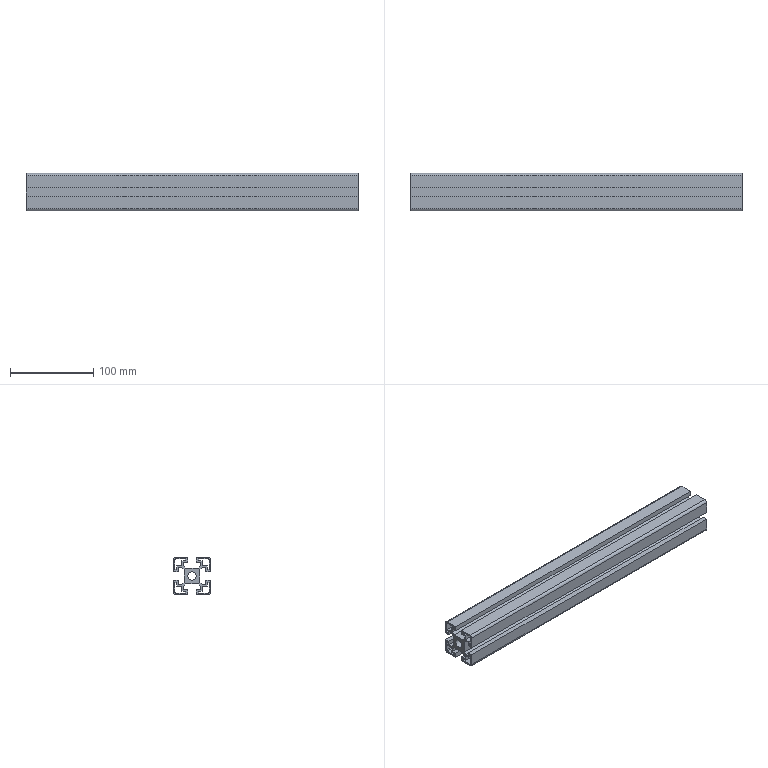Part | STEP file | 1_5 | 1 solid | 87 faces | box 400 x 45 x 45 mm | volume 327097 mm3 | plane 78 | cylinder 9 | commonest cylinder face diameters 2 x4 6 x4 10 x1